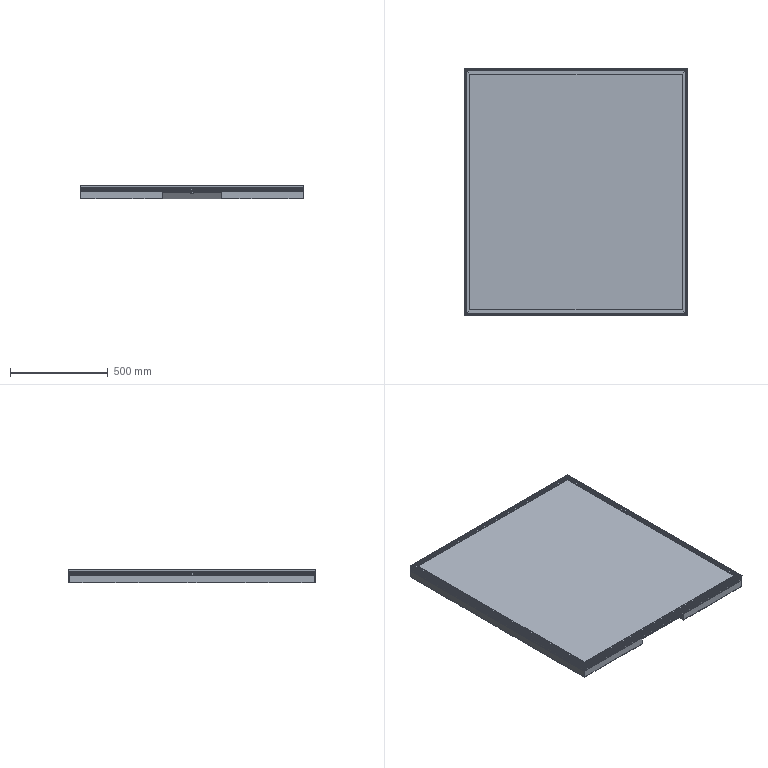Part | SolidWorks | 9 solids | 878 faces | box 1140 x 1260 x 70 mm | volume 26807789 mm3 | plane 582 | cylinder 264 | spline 32 | commonest cylinder face diameters 7 x100 0.4 x67 2.4 x41 11 x32 2 x16 1 x8